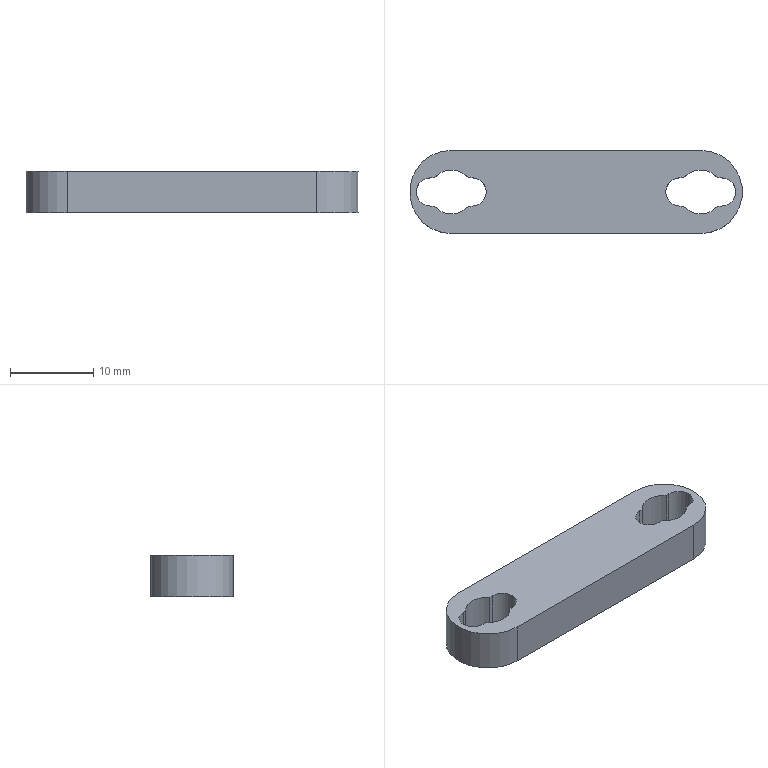Part | NX | features BREP 1 | 1 solid | 22 faces | box 40 x 10 x 5 mm | volume 1578 mm3 | plane 12 | cylinder 10 | commonest cylinder face diameters 3.4 x4 5.3 x4 10 x2
STEP:
#1=CARTESIAN_POINT('',(17.5,1.7,-2.5));
#2=VERTEX_POINT('',#1);
#3=CARTESIAN_POINT('',(17.5,-1.7,-2.5));
#4=VERTEX_POINT('',#3);
#5=CARTESIAN_POINT('',(17.5,0.,-2.5));
#6=DIRECTION('',(0.,0.,-1.));
#7=DIRECTION('',(-1.,0.,0.));
#8=AXIS2_PLACEMENT_3D('',#5,#6,#7);
#9=CIRCLE('',#8,1.7);
#10=EDGE_CURVE('',#2,#4,#9,.T.);
#11=ORIENTED_EDGE('',*,*,#10,.T.);
#12=CARTESIAN_POINT('',(17.5,-1.7,2.5));
#13=VERTEX_POINT('',#12);
#14=CARTESIAN_POINT('',(17.5,-1.7,-2.5));
#15=DIRECTION('',(0.,0.,1.));
#16=VECTOR('',#15,1000.);
#17=LINE('',#14,#16);
#18=EDGE_CURVE('',#4,#13,#17,.T.);
#19=ORIENTED_EDGE('',*,*,#18,.T.);
#20=CARTESIAN_POINT('',(17.5,1.7,2.5));
#21=VERTEX_POINT('',#20);
#22=CARTESIAN_POINT('',(17.5,0.,2.5));
#23=DIRECTION('',(0.,0.,-1.));
#24=DIRECTION('',(-1.,0.,0.));
#25=AXIS2_PLACEMENT_3D('',#22,#23,#24);
#26=CIRCLE('',#25,1.7);
#27=EDGE_CURVE('',#21,#13,#26,.T.);
#28=ORIENTED_EDGE('',*,*,#27,.F.);
#29=CARTESIAN_POINT('',(17.5,1.7,-2.5));
#30=DIRECTION('',(0.,0.,1.));
#31=VECTOR('',#30,1000.);
#32=LINE('',#29,#31);
#33=EDGE_CURVE('',#2,#21,#32,.T.);
#34=ORIENTED_EDGE('',*,*,#33,.F.);
#35=EDGE_LOOP('',(#11,#19,#28,#34));
#36=FACE_BOUND('',#35,.T.);
#37=CARTESIAN_POINT('',(17.5,0.,-2.5));
#38=DIRECTION('',(0.,0.,1.));
#39=DIRECTION('',(-1.,0.,0.));
#40=AXIS2_PLACEMENT_3D('',#37,#38,#39);
#41=CYLINDRICAL_SURFACE('',#40,1.7);
#42=ADVANCED_FACE('',(#36),#41,.F.);
#43=CARTESIAN_POINT('',(-12.5,-1.7,-2.5));
#44=VERTEX_POINT('',#43);
#45=CARTESIAN_POINT('',(-12.5,1.7,-2.5));
#46=VERTEX_POINT('',#45);
#47=CARTESIAN_POINT('',(-12.5,0.,-2.5));
#48=DIRECTION('',(0.,0.,1.));
#49=DIRECTION('',(1.,0.,0.));
#50=AXIS2_PLACEMENT_3D('',#47,#48,#49);
#51=CIRCLE('',#50,1.7);
#52=EDGE_CURVE('',#44,#46,#51,.T.);
#53=ORIENTED_EDGE('',*,*,#52,.F.);
#54=CARTESIAN_POINT('',(-12.5,-1.7,2.5));
#55=VERTEX_POINT('',#54);
#56=CARTESIAN_POINT('',(-12.5,-1.7,-2.5));
#57=DIRECTION('',(0.,0.,1.));
#58=VECTOR('',#57,1000.);
#59=LINE('',#56,#58);
#60=EDGE_CURVE('',#44,#55,#59,.T.);
#61=ORIENTED_EDGE('',*,*,#60,.T.);
#62=CARTESIAN_POINT('',(-12.5,1.7,2.5));
#63=VERTEX_POINT('',#62);
#64=CARTESIAN_POINT('',(-12.5,0.,2.5));
#65=DIRECTION('',(0.,0.,1.));
#66=DIRECTION('',(1.,0.,0.));
#67=AXIS2_PLACEMENT_3D('',#64,#65,#66);
#68=CIRCLE('',#67,1.7);
#69=EDGE_CURVE('',#55,#63,#68,.T.);
#70=ORIENTED_EDGE('',*,*,#69,.T.);
#71=CARTESIAN_POINT('',(-12.5,1.7,-2.5));
#72=DIRECTION('',(0.,0.,1.));
#73=VECTOR('',#72,1000.);
#74=LINE('',#71,#73);
#75=EDGE_CURVE('',#46,#63,#74,.T.);
#76=ORIENTED_EDGE('',*,*,#75,.F.);
#77=EDGE_LOOP('',(#53,#61,#70,#76));
#78=FACE_BOUND('',#77,.T.);
#79=CARTESIAN_POINT('',(-12.5,0.,-2.5));
#80=DIRECTION('',(0.,0.,1.));
#81=DIRECTION('',(-1.,0.,0.));
#82=AXIS2_PLACEMENT_3D('',#79,#80,#81);
#83=CYLINDRICAL_SURFACE('',#82,1.7);
#84=ADVANCED_FACE('',(#78),#83,.F.);
#85=CARTESIAN_POINT('',(-15.,5.,2.5));
#86=VERTEX_POINT('',#85);
#87=CARTESIAN_POINT('',(-15.,-5.,2.5));
#88=VERTEX_POINT('',#87);
#89=CARTESIAN_POINT('',(-15.,0.,2.5));
#90=DIRECTION('',(0.,0.,1.));
#91=DIRECTION('',(1.,0.,0.));
#92=AXIS2_PLACEMENT_3D('',#89,#90,#91);
#93=CIRCLE('',#92,5.);
#94=EDGE_CURVE('',#86,#88,#93,.T.);
#95=ORIENTED_EDGE('',*,*,#94,.F.);
#96=CARTESIAN_POINT('',(-15.,5.,-2.5));
#97=VERTEX_POINT('',#96);
#98=CARTESIAN_POINT('',(-15.,5.,2.5));
#99=DIRECTION('',(0.,0.,-1.));
#100=VECTOR('',#99,1000.);
#101=LINE('',#98,#100);
#102=EDGE_CURVE('',#86,#97,#101,.T.);
#103=ORIENTED_EDGE('',*,*,#102,.T.);
#104=CARTESIAN_POINT('',(-15.,-5.,-2.5));
#105=VERTEX_POINT('',#104);
#106=CARTESIAN_POINT('',(-15.,0.,-2.5));
#107=DIRECTION('',(0.,0.,1.));
#108=DIRECTION('',(1.,0.,0.));
#109=AXIS2_PLACEMENT_3D('',#106,#107,#108);
#110=CIRCLE('',#109,5.);
#111=EDGE_CURVE('',#97,#105,#110,.T.);
#112=ORIENTED_EDGE('',*,*,#111,.T.);
#113=CARTESIAN_POINT('',(-15.,-5.,2.5));
#114=DIRECTION('',(0.,0.,-1.));
#115=VECTOR('',#114,1000.);
#116=LINE('',#113,#115);
#117=EDGE_CURVE('',#88,#105,#116,.T.);
#118=ORIENTED_EDGE('',*,*,#117,.F.);
#119=EDGE_LOOP('',(#95,#103,#112,#118));
#120=FACE_BOUND('',#119,.T.);
#121=CARTESIAN_POINT('',(-15.,0.,2.5));
#122=DIRECTION('',(0.,0.,-1.));
#123=DIRECTION('',(1.,0.,0.));
#124=AXIS2_PLACEMENT_3D('',#121,#122,#123);
#125=CYLINDRICAL_SURFACE('',#124,5.);
#126=ADVANCED_FACE('',(#120),#125,.T.);
#127=CARTESIAN_POINT('',(-17.033,1.7,2.5));
#128=VERTEX_POINT('',#127);
#129=CARTESIAN_POINT('',(-17.5,1.7,2.5));
#130=VERTEX_POINT('',#129);
#131=CARTESIAN_POINT('',(-17.5,1.7,2.5));
#132=DIRECTION('',(-1.,0.,0.));
#133=VECTOR('',#132,1000.);
#134=LINE('',#131,#133);
#135=EDGE_CURVE('',#128,#130,#134,.T.);
#136=ORIENTED_EDGE('',*,*,#135,.F.);
#137=CARTESIAN_POINT('',(-12.967,1.7,2.5));
#138=VERTEX_POINT('',#137);
#139=CARTESIAN_POINT('',(-15.,0.,2.5));
#140=DIRECTION('',(0.,0.,1.));
#141=DIRECTION('',(1.,0.,0.));
#142=AXIS2_PLACEMENT_3D('',#139,#140,#141);
#143=CIRCLE('',#142,2.65);
#144=EDGE_CURVE('',#138,#128,#143,.T.);
#145=ORIENTED_EDGE('',*,*,#144,.F.);
#146=CARTESIAN_POINT('',(-17.5,1.7,2.5));
#147=DIRECTION('',(-1.,0.,0.));
#148=VECTOR('',#147,1000.);
#149=LINE('',#146,#148);
#150=EDGE_CURVE('',#63,#138,#149,.T.);
#151=ORIENTED_EDGE('',*,*,#150,.F.);
#152=ORIENTED_EDGE('',*,*,#69,.F.);
#153=CARTESIAN_POINT('',(-12.967,-1.7,2.5));
#154=VERTEX_POINT('',#153);
#155=CARTESIAN_POINT('',(-17.5,-1.7,2.5));
#156=DIRECTION('',(1.,0.,0.));
#157=VECTOR('',#156,1000.);
#158=LINE('',#155,#157);
#159=EDGE_CURVE('',#154,#55,#158,.T.);
#160=ORIENTED_EDGE('',*,*,#159,.F.);
#161=CARTESIAN_POINT('',(-17.033,-1.7,2.5));
#162=VERTEX_POINT('',#161);
#163=CARTESIAN_POINT('',(-15.,0.,2.5));
#164=DIRECTION('',(0.,0.,1.));
#165=DIRECTION('',(1.,0.,0.));
#166=AXIS2_PLACEMENT_3D('',#163,#164,#165);
#167=CIRCLE('',#166,2.65);
#168=EDGE_CURVE('',#162,#154,#167,.T.);
#169=ORIENTED_EDGE('',*,*,#168,.F.);
#170=CARTESIAN_POINT('',(-17.5,-1.7,2.5));
#171=VERTEX_POINT('',#170);
#172=CARTESIAN_POINT('',(-17.5,-1.7,2.5));
#173=DIRECTION('',(1.,0.,0.));
#174=VECTOR('',#173,1000.);
#175=LINE('',#172,#174);
#176=EDGE_CURVE('',#171,#162,#175,.T.);
#177=ORIENTED_EDGE('',*,*,#176,.F.);
#178=CARTESIAN_POINT('',(-17.5,0.,2.5));
#179=DIRECTION('',(0.,0.,1.));
#180=DIRECTION('',(1.,0.,0.));
#181=AXIS2_PLACEMENT_3D('',#178,#179,#180);
#182=CIRCLE('',#181,1.7);
#183=EDGE_CURVE('',#130,#171,#182,.T.);
#184=ORIENTED_EDGE('',*,*,#183,.F.);
#185=EDGE_LOOP('',(#136,#145,#151,#152,#160,#169,#177,#184));
#186=FACE_BOUND('',#185,.T.);
#187=CARTESIAN_POINT('',(15.,5.,2.5));
#188=VERTEX_POINT('',#187);
#189=CARTESIAN_POINT('',(-15.,5.,2.5));
#190=DIRECTION('',(-1.,0.,0.));
#191=VECTOR('',#190,1000.);
#192=LINE('',#189,#191);
#193=EDGE_CURVE('',#188,#86,#192,.T.);
#194=ORIENTED_EDGE('',*,*,#193,.T.);
#195=ORIENTED_EDGE('',*,*,#94,.T.);
#196=CARTESIAN_POINT('',(15.,-5.,2.5));
#197=VERTEX_POINT('',#196);
#198=CARTESIAN_POINT('',(-15.,-5.,2.5));
#199=DIRECTION('',(1.,0.,0.));
#200=VECTOR('',#199,1000.);
#201=LINE('',#198,#200);
#202=EDGE_CURVE('',#88,#197,#201,.T.);
#203=ORIENTED_EDGE('',*,*,#202,.T.);
#204=CARTESIAN_POINT('',(15.,0.,2.5));
#205=DIRECTION('',(0.,0.,1.));
#206=DIRECTION('',(1.,0.,0.));
#207=AXIS2_PLACEMENT_3D('',#204,#205,#206);
#208=CIRCLE('',#207,5.);
#209=EDGE_CURVE('',#197,#188,#208,.T.);
#210=ORIENTED_EDGE('',*,*,#209,.T.);
#211=EDGE_LOOP('',(#194,#195,#203,#210));
#212=FACE_BOUND('',#211,.T.);
#213=CARTESIAN_POINT('',(12.967,-1.7,2.5));
#214=VERTEX_POINT('',#213);
#215=CARTESIAN_POINT('',(17.033,-1.7,2.5));
#216=VERTEX_POINT('',#215);
#217=CARTESIAN_POINT('',(15.,0.,2.5));
#218=DIRECTION('',(0.,0.,1.));
#219=DIRECTION('',(1.,0.,0.));
#220=AXIS2_PLACEMENT_3D('',#217,#218,#219);
#221=CIRCLE('',#220,2.65);
#222=EDGE_CURVE('',#214,#216,#221,.T.);
#223=ORIENTED_EDGE('',*,*,#222,.F.);
#224=CARTESIAN_POINT('',(12.5,-1.7,2.5));
#225=VERTEX_POINT('',#224);
#226=CARTESIAN_POINT('',(17.5,-1.7,2.5));
#227=DIRECTION('',(-1.,0.,0.));
#228=VECTOR('',#227,1000.);
#229=LINE('',#226,#228);
#230=EDGE_CURVE('',#214,#225,#229,.T.);
#231=ORIENTED_EDGE('',*,*,#230,.T.);
#232=CARTESIAN_POINT('',(12.5,1.7,2.5));
#233=VERTEX_POINT('',#232);
#234=CARTESIAN_POINT('',(12.5,0.,2.5));
#235=DIRECTION('',(0.,0.,-1.));
#236=DIRECTION('',(-1.,0.,0.));
#237=AXIS2_PLACEMENT_3D('',#234,#235,#236);
#238=CIRCLE('',#237,1.7);
#239=EDGE_CURVE('',#225,#233,#238,.T.);
#240=ORIENTED_EDGE('',*,*,#239,.T.);
#241=CARTESIAN_POINT('',(12.967,1.7,2.5));
#242=VERTEX_POINT('',#241);
#243=CARTESIAN_POINT('',(17.5,1.7,2.5));
#244=DIRECTION('',(1.,0.,0.));
#245=VECTOR('',#244,1000.);
#246=LINE('',#243,#245);
#247=EDGE_CURVE('',#233,#242,#246,.T.);
#248=ORIENTED_EDGE('',*,*,#247,.T.);
#249=CARTESIAN_POINT('',(17.033,1.7,2.5));
#250=VERTEX_POINT('',#249);
#251=CARTESIAN_POINT('',(15.,0.,2.5));
#252=DIRECTION('',(0.,0.,1.));
#253=DIRECTION('',(1.,0.,0.));
#254=AXIS2_PLACEMENT_3D('',#251,#252,#253);
#255=CIRCLE('',#254,2.65);
#256=EDGE_CURVE('',#250,#242,#255,.T.);
#257=ORIENTED_EDGE('',*,*,#256,.F.);
#258=CARTESIAN_POINT('',(17.5,1.7,2.5));
#259=DIRECTION('',(1.,0.,0.));
#260=VECTOR('',#259,1000.);
#261=LINE('',#258,#260);
#262=EDGE_CURVE('',#250,#21,#261,.T.);
#263=ORIENTED_EDGE('',*,*,#262,.T.);
#264=ORIENTED_EDGE('',*,*,#27,.T.);
#265=CARTESIAN_POINT('',(17.5,-1.7,2.5));
#266=DIRECTION('',(-1.,0.,0.));
#267=VECTOR('',#266,1000.);
#268=LINE('',#265,#267);
#269=EDGE_CURVE('',#13,#216,#268,.T.);
#270=ORIENTED_EDGE('',*,*,#269,.T.);
#271=EDGE_LOOP('',(#223,#231,#240,#248,#257,#263,#264,#270));
#272=FACE_BOUND('',#271,.T.);
#273=CARTESIAN_POINT('',(-15.,0.,2.5));
#274=DIRECTION('',(0.,0.,1.));
#275=DIRECTION('',(-1.,0.,0.));
#276=AXIS2_PLACEMENT_3D('',#273,#274,#275);
#277=PLANE('',#276);
#278=ADVANCED_FACE('',(#186,#212,#272),#277,.T.);
#279=CARTESIAN_POINT('',(-12.967,1.7,-2.5));
#280=VERTEX_POINT('',#279);
#281=CARTESIAN_POINT('',(-17.033,1.7,-2.5));
#282=VERTEX_POINT('',#281);
#283=CARTESIAN_POINT('',(-15.,0.,-2.5));
#284=DIRECTION('',(0.,0.,1.));
#285=DIRECTION('',(1.,0.,0.));
#286=AXIS2_PLACEMENT_3D('',#283,#284,#285);
#287=CIRCLE('',#286,2.65);
#288=EDGE_CURVE('',#280,#282,#287,.T.);
#289=ORIENTED_EDGE('',*,*,#288,.T.);
#290=CARTESIAN_POINT('',(-17.5,1.7,-2.5));
#291=VERTEX_POINT('',#290);
#292=CARTESIAN_POINT('',(-17.5,1.7,-2.5));
#293=DIRECTION('',(-1.,0.,0.));
#294=VECTOR('',#293,1000.);
#295=LINE('',#292,#294);
#296=EDGE_CURVE('',#282,#291,#295,.T.);
#297=ORIENTED_EDGE('',*,*,#296,.T.);
#298=CARTESIAN_POINT('',(-17.5,-1.7,-2.5));
#299=VERTEX_POINT('',#298);
#300=CARTESIAN_POINT('',(-17.5,0.,-2.5));
#301=DIRECTION('',(0.,0.,1.));
#302=DIRECTION('',(1.,0.,0.));
#303=AXIS2_PLACEMENT_3D('',#300,#301,#302);
#304=CIRCLE('',#303,1.7);
#305=EDGE_CURVE('',#291,#299,#304,.T.);
#306=ORIENTED_EDGE('',*,*,#305,.T.);
#307=CARTESIAN_POINT('',(-17.033,-1.7,-2.5));
#308=VERTEX_POINT('',#307);
#309=CARTESIAN_POINT('',(-17.5,-1.7,-2.5));
#310=DIRECTION('',(1.,0.,0.));
#311=VECTOR('',#310,1000.);
#312=LINE('',#309,#311);
#313=EDGE_CURVE('',#299,#308,#312,.T.);
#314=ORIENTED_EDGE('',*,*,#313,.T.);
#315=CARTESIAN_POINT('',(-12.967,-1.7,-2.5));
#316=VERTEX_POINT('',#315);
#317=CARTESIAN_POINT('',(-15.,0.,-2.5));
#318=DIRECTION('',(0.,0.,1.));
#319=DIRECTION('',(1.,0.,0.));
#320=AXIS2_PLACEMENT_3D('',#317,#318,#319);
#321=CIRCLE('',#320,2.65);
#322=EDGE_CURVE('',#308,#316,#321,.T.);
#323=ORIENTED_EDGE('',*,*,#322,.T.);
#324=CARTESIAN_POINT('',(-17.5,-1.7,-2.5));
#325=DIRECTION('',(1.,0.,0.));
#326=VECTOR('',#325,1000.);
#327=LINE('',#324,#326);
#328=EDGE_CURVE('',#316,#44,#327,.T.);
#329=ORIENTED_EDGE('',*,*,#328,.T.);
#330=ORIENTED_EDGE('',*,*,#52,.T.);
#331=CARTESIAN_POINT('',(-17.5,1.7,-2.5));
#332=DIRECTION('',(-1.,0.,0.));
#333=VECTOR('',#332,1000.);
#334=LINE('',#331,#333);
#335=EDGE_CURVE('',#46,#280,#334,.T.);
#336=ORIENTED_EDGE('',*,*,#335,.T.);
#337=EDGE_LOOP('',(#289,#297,#306,#314,#323,#329,#330,#336));
#338=FACE_BOUND('',#337,.T.);
#339=ORIENTED_EDGE('',*,*,#111,.F.);
#340=CARTESIAN_POINT('',(15.,5.,-2.5));
#341=VERTEX_POINT('',#340);
#342=CARTESIAN_POINT('',(-15.,5.,-2.5));
#343=DIRECTION('',(-1.,0.,0.));
#344=VECTOR('',#343,1000.);
#345=LINE('',#342,#344);
#346=EDGE_CURVE('',#341,#97,#345,.T.);
#347=ORIENTED_EDGE('',*,*,#346,.F.);
#348=CARTESIAN_POINT('',(15.,-5.,-2.5));
#349=VERTEX_POINT('',#348);
#350=CARTESIAN_POINT('',(15.,0.,-2.5));
#351=DIRECTION('',(0.,0.,1.));
#352=DIRECTION('',(1.,0.,0.));
#353=AXIS2_PLACEMENT_3D('',#350,#351,#352);
#354=CIRCLE('',#353,5.);
#355=EDGE_CURVE('',#349,#341,#354,.T.);
#356=ORIENTED_EDGE('',*,*,#355,.F.);
#357=CARTESIAN_POINT('',(-15.,-5.,-2.5));
#358=DIRECTION('',(1.,0.,0.));
#359=VECTOR('',#358,1000.);
#360=LINE('',#357,#359);
#361=EDGE_CURVE('',#105,#349,#360,.T.);
#362=ORIENTED_EDGE('',*,*,#361,.F.);
#363=EDGE_LOOP('',(#339,#347,#356,#362));
#364=FACE_BOUND('',#363,.T.);
#365=CARTESIAN_POINT('',(12.967,-1.7,-2.5));
#366=VERTEX_POINT('',#365);
#367=CARTESIAN_POINT('',(12.5,-1.7,-2.5));
#368=VERTEX_POINT('',#367);
#369=CARTESIAN_POINT('',(17.5,-1.7,-2.5));
#370=DIRECTION('',(-1.,0.,0.));
#371=VECTOR('',#370,1000.);
#372=LINE('',#369,#371);
#373=EDGE_CURVE('',#366,#368,#372,.T.);
#374=ORIENTED_EDGE('',*,*,#373,.F.);
#375=CARTESIAN_POINT('',(17.033,-1.7,-2.5));
#376=VERTEX_POINT('',#375);
#377=CARTESIAN_POINT('',(15.,0.,-2.5));
#378=DIRECTION('',(0.,0.,1.));
#379=DIRECTION('',(1.,0.,0.));
#380=AXIS2_PLACEMENT_3D('',#377,#378,#379);
#381=CIRCLE('',#380,2.65);
#382=EDGE_CURVE('',#366,#376,#381,.T.);
#383=ORIENTED_EDGE('',*,*,#382,.T.);
#384=CARTESIAN_POINT('',(17.5,-1.7,-2.5));
#385=DIRECTION('',(-1.,0.,0.));
#386=VECTOR('',#385,1000.);
#387=LINE('',#384,#386);
#388=EDGE_CURVE('',#4,#376,#387,.T.);
#389=ORIENTED_EDGE('',*,*,#388,.F.);
#390=ORIENTED_EDGE('',*,*,#10,.F.);
#391=CARTESIAN_POINT('',(17.033,1.7,-2.5));
#392=VERTEX_POINT('',#391);
#393=CARTESIAN_POINT('',(17.5,1.7,-2.5));
#394=DIRECTION('',(1.,0.,0.));
#395=VECTOR('',#394,1000.);
#396=LINE('',#393,#395);
#397=EDGE_CURVE('',#392,#2,#396,.T.);
#398=ORIENTED_EDGE('',*,*,#397,.F.);
#399=CARTESIAN_POINT('',(12.967,1.7,-2.5));
#400=VERTEX_POINT('',#399);
#401=CARTESIAN_POINT('',(15.,0.,-2.5));
#402=DIRECTION('',(0.,0.,1.));
#403=DIRECTION('',(1.,0.,0.));
#404=AXIS2_PLACEMENT_3D('',#401,#402,#403);
#405=CIRCLE('',#404,2.65);
#406=EDGE_CURVE('',#392,#400,#405,.T.);
#407=ORIENTED_EDGE('',*,*,#406,.T.);
#408=CARTESIAN_POINT('',(12.5,1.7,-2.5));
#409=VERTEX_POINT('',#408);
#410=CARTESIAN_POINT('',(17.5,1.7,-2.5));
#411=DIRECTION('',(1.,0.,0.));
#412=VECTOR('',#411,1000.);
#413=LINE('',#410,#412);
#414=EDGE_CURVE('',#409,#400,#413,.T.);
#415=ORIENTED_EDGE('',*,*,#414,.F.);
#416=CARTESIAN_POINT('',(12.5,0.,-2.5));
#417=DIRECTION('',(0.,0.,-1.));
#418=DIRECTION('',(-1.,0.,0.));
#419=AXIS2_PLACEMENT_3D('',#416,#417,#418);
#420=CIRCLE('',#419,1.7);
#421=EDGE_CURVE('',#368,#409,#420,.T.);
#422=ORIENTED_EDGE('',*,*,#421,.F.);
#423=EDGE_LOOP('',(#374,#383,#389,#390,#398,#407,#415,#422));
#424=FACE_BOUND('',#423,.T.);
#425=CARTESIAN_POINT('',(-15.,0.,-2.5));
#426=DIRECTION('',(0.,0.,1.));
#427=DIRECTION('',(-1.,0.,0.));
#428=AXIS2_PLACEMENT_3D('',#425,#426,#427);
#429=PLANE('',#428);
#430=ADVANCED_FACE('',(#338,#364,#424),#429,.F.);
#431=CARTESIAN_POINT('',(12.967,-1.7,-2.5));
#432=DIRECTION('',(0.,0.,-1.));
#433=VECTOR('',#432,1000.);
#434=LINE('',#431,#433);
#435=EDGE_CURVE('',#214,#366,#434,.T.);
#436=ORIENTED_EDGE('',*,*,#435,.F.);
#437=ORIENTED_EDGE('',*,*,#222,.T.);
#438=CARTESIAN_POINT('',(17.033,-1.7,-2.5));
#439=DIRECTION('',(0.,0.,1.));
#440=VECTOR('',#439,1000.);
#441=LINE('',#438,#440);
#442=EDGE_CURVE('',#376,#216,#441,.T.);
#443=ORIENTED_EDGE('',*,*,#442,.F.);
#444=ORIENTED_EDGE('',*,*,#382,.F.);
#445=EDGE_LOOP('',(#436,#437,#443,#444));
#446=FACE_BOUND('',#445,.T.);
#447=CARTESIAN_POINT('',(15.,0.,-2.5));
#448=DIRECTION('',(0.,0.,1.));
#449=DIRECTION('',(-1.,0.,0.));
#450=AXIS2_PLACEMENT_3D('',#447,#448,#449);
#451=CYLINDRICAL_SURFACE('',#450,2.65);
#452=ADVANCED_FACE('',(#446),#451,.F.);
#453=CARTESIAN_POINT('',(17.033,1.7,-2.5));
#454=DIRECTION('',(0.,0.,-1.));
#455=VECTOR('',#454,1000.);
#456=LINE('',#453,#455);
#457=EDGE_CURVE('',#250,#392,#456,.T.);
#458=ORIENTED_EDGE('',*,*,#457,.F.);
#459=ORIENTED_EDGE('',*,*,#256,.T.);
#460=CARTESIAN_POINT('',(12.967,1.7,-2.5));
#461=DIRECTION('',(0.,0.,1.));
#462=VECTOR('',#461,1000.);
#463=LINE('',#460,#462);
#464=EDGE_CURVE('',#400,#242,#463,.T.);
#465=ORIENTED_EDGE('',*,*,#464,.F.);
#466=ORIENTED_EDGE('',*,*,#406,.F.);
#467=EDGE_LOOP('',(#458,#459,#465,#466));
#468=FACE_BOUND('',#467,.T.);
#469=CARTESIAN_POINT('',(15.,0.,-2.5));
#470=DIRECTION('',(0.,0.,1.));
#471=DIRECTION('',(-1.,0.,0.));
#472=AXIS2_PLACEMENT_3D('',#469,#470,#471);
#473=CYLINDRICAL_SURFACE('',#472,2.65);
#474=ADVANCED_FACE('',(#468),#473,.F.);
#475=ORIENTED_EDGE('',*,*,#144,.T.);
#476=CARTESIAN_POINT('',(-17.033,1.7,-2.5));
#477=DIRECTION('',(0.,0.,-1.));
#478=VECTOR('',#477,1000.);
#479=LINE('',#476,#478);
#480=EDGE_CURVE('',#128,#282,#479,.T.);
#481=ORIENTED_EDGE('',*,*,#480,.T.);
#482=ORIENTED_EDGE('',*,*,#288,.F.);
#483=CARTESIAN_POINT('',(-12.967,1.7,-2.5));
#484=DIRECTION('',(0.,0.,1.));
#485=VECTOR('',#484,1000.);
#486=LINE('',#483,#485);
#487=EDGE_CURVE('',#280,#138,#486,.T.);
#488=ORIENTED_EDGE('',*,*,#487,.T.);
#489=EDGE_LOOP('',(#475,#481,#482,#488));
#490=FACE_BOUND('',#489,.T.);
#491=CARTESIAN_POINT('',(-15.,0.,-2.5));
#492=DIRECTION('',(0.,0.,1.));
#493=DIRECTION('',(-1.,0.,0.));
#494=AXIS2_PLACEMENT_3D('',#491,#492,#493);
#495=CYLINDRICAL_SURFACE('',#494,2.65);
#496=ADVANCED_FACE('',(#490),#495,.F.);
#497=ORIENTED_EDGE('',*,*,#361,.T.);
#498=CARTESIAN_POINT('',(15.,-5.,2.5));
#499=DIRECTION('',(0.,0.,-1.));
#500=VECTOR('',#499,1000.);
#501=LINE('',#498,#500);
#502=EDGE_CURVE('',#197,#349,#501,.T.);
#503=ORIENTED_EDGE('',*,*,#502,.F.);
#504=ORIENTED_EDGE('',*,*,#202,.F.);
#505=ORIENTED_EDGE('',*,*,#117,.T.);
#506=EDGE_LOOP('',(#497,#503,#504,#505));
#507=FACE_BOUND('',#506,.T.);
#508=CARTESIAN_POINT('',(-15.,-5.,2.5));
#509=DIRECTION('',(0.,1.,0.));
#510=DIRECTION('',(0.,0.,-1.));
#511=AXIS2_PLACEMENT_3D('',#508,#509,#510);
#512=PLANE('',#511);
#513=ADVANCED_FACE('',(#507),#512,.F.);
#514=ORIENTED_EDGE('',*,*,#355,.T.);
#515=CARTESIAN_POINT('',(15.,5.,2.5));
#516=DIRECTION('',(0.,0.,-1.));
#517=VECTOR('',#516,1000.);
#518=LINE('',#515,#517);
#519=EDGE_CURVE('',#188,#341,#518,.T.);
#520=ORIENTED_EDGE('',*,*,#519,.F.);
#521=ORIENTED_EDGE('',*,*,#209,.F.);
#522=ORIENTED_EDGE('',*,*,#502,.T.);
#523=EDGE_LOOP('',(#514,#520,#521,#522));
#524=FACE_BOUND('',#523,.T.);
#525=CARTESIAN_POINT('',(15.,0.,2.5));
#526=DIRECTION('',(0.,0.,-1.));
#527=DIRECTION('',(1.,0.,0.));
#528=AXIS2_PLACEMENT_3D('',#525,#526,#527);
#529=CYLINDRICAL_SURFACE('',#528,5.);
#530=ADVANCED_FACE('',(#524),#529,.T.);
#531=ORIENTED_EDGE('',*,*,#346,.T.);
#532=ORIENTED_EDGE('',*,*,#102,.F.);
#533=ORIENTED_EDGE('',*,*,#193,.F.);
#534=ORIENTED_EDGE('',*,*,#519,.T.);
#535=EDGE_LOOP('',(#531,#532,#533,#534));
#536=FACE_BOUND('',#535,.T.);
#537=CARTESIAN_POINT('',(-15.,5.,2.5));
#538=DIRECTION('',(0.,-1.,0.));
#539=DIRECTION('',(-1.,0.,0.));
#540=AXIS2_PLACEMENT_3D('',#537,#538,#539);
#541=PLANE('',#540);
#542=ADVANCED_FACE('',(#536),#541,.F.);
#543=ORIENTED_EDGE('',*,*,#168,.T.);
#544=CARTESIAN_POINT('',(-12.967,-1.7,-2.5));
#545=DIRECTION('',(0.,0.,-1.));
#546=VECTOR('',#545,1000.);
#547=LINE('',#544,#546);
#548=EDGE_CURVE('',#154,#316,#547,.T.);
#549=ORIENTED_EDGE('',*,*,#548,.T.);
#550=ORIENTED_EDGE('',*,*,#322,.F.);
#551=CARTESIAN_POINT('',(-17.033,-1.7,-2.5));
#552=DIRECTION('',(0.,0.,1.));
#553=VECTOR('',#552,1000.);
#554=LINE('',#551,#553);
#555=EDGE_CURVE('',#308,#162,#554,.T.);
#556=ORIENTED_EDGE('',*,*,#555,.T.);
#557=EDGE_LOOP('',(#543,#549,#550,#556));
#558=FACE_BOUND('',#557,.T.);
#559=CARTESIAN_POINT('',(-15.,0.,-2.5));
#560=DIRECTION('',(0.,0.,1.));
#561=DIRECTION('',(-1.,0.,0.));
#562=AXIS2_PLACEMENT_3D('',#559,#560,#561);
#563=CYLINDRICAL_SURFACE('',#562,2.65);
#564=ADVANCED_FACE('',(#558),#563,.F.);
#565=ORIENTED_EDGE('',*,*,#313,.F.);
#566=CARTESIAN_POINT('',(-17.5,-1.7,-2.5));
#567=DIRECTION('',(0.,0.,1.));
#568=VECTOR('',#567,1000.);
#569=LINE('',#566,#568);
#570=EDGE_CURVE('',#299,#171,#569,.T.);
#571=ORIENTED_EDGE('',*,*,#570,.T.);
#572=ORIENTED_EDGE('',*,*,#176,.T.);
#573=ORIENTED_EDGE('',*,*,#555,.F.);
#574=EDGE_LOOP('',(#565,#571,#572,#573));
#575=FACE_BOUND('',#574,.T.);
#576=CARTESIAN_POINT('',(-17.5,-1.7,-2.5));
#577=DIRECTION('',(0.,-1.,0.));
#578=DIRECTION('',(-1.,0.,0.));
#579=AXIS2_PLACEMENT_3D('',#576,#577,#578);
#580=PLANE('',#579);
#581=ADVANCED_FACE('',(#575),#580,.F.);
#582=ORIENTED_EDGE('',*,*,#135,.T.);
#583=CARTESIAN_POINT('',(-17.5,1.7,-2.5));
#584=DIRECTION('',(0.,0.,1.));
#585=VECTOR('',#584,1000.);
#586=LINE('',#583,#585);
#587=EDGE_CURVE('',#291,#130,#586,.T.);
#588=ORIENTED_EDGE('',*,*,#587,.F.);
#589=ORIENTED_EDGE('',*,*,#296,.F.);
#590=ORIENTED_EDGE('',*,*,#480,.F.);
#591=EDGE_LOOP('',(#582,#588,#589,#590));
#592=FACE_BOUND('',#591,.T.);
#593=CARTESIAN_POINT('',(-17.5,1.7,-2.5));
#594=DIRECTION('',(0.,1.,0.));
#595=DIRECTION('',(1.,0.,0.));
#596=AXIS2_PLACEMENT_3D('',#593,#594,#595);
#597=PLANE('',#596);
#598=ADVANCED_FACE('',(#592),#597,.F.);
#599=ORIENTED_EDGE('',*,*,#183,.T.);
#600=ORIENTED_EDGE('',*,*,#570,.F.);
#601=ORIENTED_EDGE('',*,*,#305,.F.);
#602=ORIENTED_EDGE('',*,*,#587,.T.);
#603=EDGE_LOOP('',(#599,#600,#601,#602));
#604=FACE_BOUND('',#603,.T.);
#605=CARTESIAN_POINT('',(-17.5,0.,-2.5));
#606=DIRECTION('',(0.,0.,1.));
#607=DIRECTION('',(-1.,0.,0.));
#608=AXIS2_PLACEMENT_3D('',#605,#606,#607);
#609=CYLINDRICAL_SURFACE('',#608,1.7);
#610=ADVANCED_FACE('',(#604),#609,.F.);
#611=ORIENTED_EDGE('',*,*,#335,.F.);
#612=ORIENTED_EDGE('',*,*,#75,.T.);
#613=ORIENTED_EDGE('',*,*,#150,.T.);
#614=ORIENTED_EDGE('',*,*,#487,.F.);
#615=EDGE_LOOP('',(#611,#612,#613,#614));
#616=FACE_BOUND('',#615,.T.);
#617=CARTESIAN_POINT('',(-17.5,1.7,-2.5));
#618=DIRECTION('',(0.,1.,0.));
#619=DIRECTION('',(1.,0.,0.));
#620=AXIS2_PLACEMENT_3D('',#617,#618,#619);
#621=PLANE('',#620);
#622=ADVANCED_FACE('',(#616),#621,.F.);
#623=ORIENTED_EDGE('',*,*,#159,.T.);
#624=ORIENTED_EDGE('',*,*,#60,.F.);
#625=ORIENTED_EDGE('',*,*,#328,.F.);
#626=ORIENTED_EDGE('',*,*,#548,.F.);
#627=EDGE_LOOP('',(#623,#624,#625,#626));
#628=FACE_BOUND('',#627,.T.);
#629=CARTESIAN_POINT('',(-17.5,-1.7,-2.5));
#630=DIRECTION('',(0.,-1.,0.));
#631=DIRECTION('',(-1.,0.,0.));
#632=AXIS2_PLACEMENT_3D('',#629,#630,#631);
#633=PLANE('',#632);
#634=ADVANCED_FACE('',(#628),#633,.F.);
#635=ORIENTED_EDGE('',*,*,#435,.T.);
#636=ORIENTED_EDGE('',*,*,#373,.T.);
#637=CARTESIAN_POINT('',(12.5,-1.7,-2.5));
#638=DIRECTION('',(0.,0.,1.));
#639=VECTOR('',#638,1000.);
#640=LINE('',#637,#639);
#641=EDGE_CURVE('',#368,#225,#640,.T.);
#642=ORIENTED_EDGE('',*,*,#641,.T.);
#643=ORIENTED_EDGE('',*,*,#230,.F.);
#644=EDGE_LOOP('',(#635,#636,#642,#643));
#645=FACE_BOUND('',#644,.T.);
#646=CARTESIAN_POINT('',(17.5,-1.7,-2.5));
#647=DIRECTION('',(0.,1.,0.));
#648=DIRECTION('',(1.,0.,0.));
#649=AXIS2_PLACEMENT_3D('',#646,#647,#648);
#650=PLANE('',#649);
#651=ADVANCED_FACE('',(#645),#650,.T.);
#652=ORIENTED_EDGE('',*,*,#464,.T.);
#653=ORIENTED_EDGE('',*,*,#247,.F.);
#654=CARTESIAN_POINT('',(12.5,1.7,-2.5));
#655=DIRECTION('',(0.,0.,1.));
#656=VECTOR('',#655,1000.);
#657=LINE('',#654,#656);
#658=EDGE_CURVE('',#409,#233,#657,.T.);
#659=ORIENTED_EDGE('',*,*,#658,.F.);
#660=ORIENTED_EDGE('',*,*,#414,.T.);
#661=EDGE_LOOP('',(#652,#653,#659,#660));
#662=FACE_BOUND('',#661,.T.);
#663=CARTESIAN_POINT('',(17.5,1.7,-2.5));
#664=DIRECTION('',(0.,-1.,0.));
#665=DIRECTION('',(-1.,0.,0.));
#666=AXIS2_PLACEMENT_3D('',#663,#664,#665);
#667=PLANE('',#666);
#668=ADVANCED_FACE('',(#662),#667,.T.);
#669=ORIENTED_EDGE('',*,*,#239,.F.);
#670=ORIENTED_EDGE('',*,*,#641,.F.);
#671=ORIENTED_EDGE('',*,*,#421,.T.);
#672=ORIENTED_EDGE('',*,*,#658,.T.);
#673=EDGE_LOOP('',(#669,#670,#671,#672));
#674=FACE_BOUND('',#673,.T.);
#675=CARTESIAN_POINT('',(12.5,0.,-2.5));
#676=DIRECTION('',(0.,0.,1.));
#677=DIRECTION('',(-1.,0.,0.));
#678=AXIS2_PLACEMENT_3D('',#675,#676,#677);
#679=CYLINDRICAL_SURFACE('',#678,1.7);
#680=ADVANCED_FACE('',(#674),#679,.F.);
#681=ORIENTED_EDGE('',*,*,#442,.T.);
#682=ORIENTED_EDGE('',*,*,#269,.F.);
#683=ORIENTED_EDGE('',*,*,#18,.F.);
#684=ORIENTED_EDGE('',*,*,#388,.T.);
#685=EDGE_LOOP('',(#681,#682,#683,#684));
#686=FACE_BOUND('',#685,.T.);
#687=CARTESIAN_POINT('',(17.5,-1.7,-2.5));
#688=DIRECTION('',(0.,1.,0.));
#689=DIRECTION('',(1.,0.,0.));
#690=AXIS2_PLACEMENT_3D('',#687,#688,#689);
#691=PLANE('',#690);
#692=ADVANCED_FACE('',(#686),#691,.T.);
#693=ORIENTED_EDGE('',*,*,#457,.T.);
#694=ORIENTED_EDGE('',*,*,#397,.T.);
#695=ORIENTED_EDGE('',*,*,#33,.T.);
#696=ORIENTED_EDGE('',*,*,#262,.F.);
#697=EDGE_LOOP('',(#693,#694,#695,#696));
#698=FACE_BOUND('',#697,.T.);
#699=CARTESIAN_POINT('',(17.5,1.7,-2.5));
#700=DIRECTION('',(0.,-1.,0.));
#701=DIRECTION('',(-1.,0.,0.));
#702=AXIS2_PLACEMENT_3D('',#699,#700,#701);
#703=PLANE('',#702);
#704=ADVANCED_FACE('',(#698),#703,.T.);
#705=CLOSED_SHELL('',(#42,#84,#126,#278,#430,#452,#474,#496,#513,#530,#542,#564,#581,#598,#610,#622,#634,#651,#668,#680,#692,#704));
#706=MANIFOLD_SOLID_BREP('',#705);
#707=(LENGTH_UNIT()NAMED_UNIT(*)SI_UNIT(.MILLI.,.METRE.));
#708=UNCERTAINTY_MEASURE_WITH_UNIT(LENGTH_MEASURE(0.00001),#707,'','');
#709=(NAMED_UNIT(*)PLANE_ANGLE_UNIT()SI_UNIT($,.RADIAN.));
#710=(NAMED_UNIT(*)SI_UNIT($,.STERADIAN.)SOLID_ANGLE_UNIT());
#711=(GEOMETRIC_REPRESENTATION_CONTEXT(3)GLOBAL_UNCERTAINTY_ASSIGNED_CONTEXT((#708))GLOBAL_UNIT_ASSIGNED_CONTEXT((#707,#709,#710))REPRESENTATION_CONTEXT('',''));
#712=ADVANCED_BREP_SHAPE_REPRESENTATION('',(#706),#711);